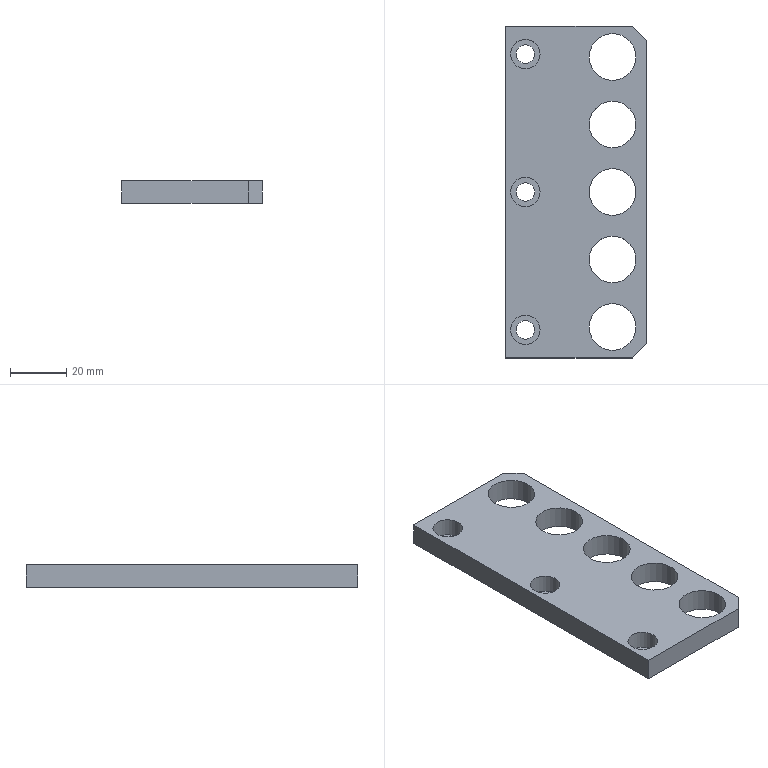NC program | NX | posted with a generic post | part box 50 x 118 x 8 mm
Whole program:
N10 G17 G21 G94 G90
(PLANAR_MILL_6 , TOOL : D63R0.8)
N12 T01 M6
N14 G54
N16 G17 G0 G90 X98.825 Y0.176 S2500 M3
N18 G43 Z30. H1
N20 Z5.7
N22 G94 G1 Z3.7 F800.
N24 X62.5
N26 X-62.5
N28 X-98.825
N30 Z5.7
N32 G0 Z30.
N34 X98.975 Y0.025
N36 Z5.4
N38 G1 Z3.4
N40 X62.5
N42 X-62.5
N44 X-98.975
N46 Z5.4
N48 G0 Z30.
N50 X99. Y0.
N52 Z5.1
N54 G1 Z3.1
N56 X62.5
N58 X-62.5
N60 X-99.
N62 Z5.1
N64 G0 Z30.
N66 X99.
N68 Z4.8
N70 G1 Z2.8
N72 X62.5
N74 X-62.5
N76 X-99.
N78 Z4.8
N80 G0 Z30.
N82 X99.
N84 Z4.5
N86 G1 Z2.5
N88 X62.5
N90 X-62.5
N92 X-99.
N94 Z4.5
N96 G0 Z30.
N98 X99.
N100 Z4.2
N102 G1 Z2.2
N104 X62.5
N106 X-62.5
N108 X-99.
N110 Z4.2
N112 G0 Z30.
N114 X99.
N116 Z3.9
N118 G1 Z1.9
N120 X62.5
N122 X-62.5
N124 X-99.
N126 Z3.9
N128 G0 Z30.
N130 X99.
N132 Z3.6
N134 G1 Z1.6
N136 X62.5
N138 X-62.5
N140 X-99.
N142 Z3.6
N144 G0 Z30.
N146 X99.
N148 Z3.3
N150 G1 Z1.3
N152 X62.5
N154 X-62.5
N156 X-99.
N158 Z3.3
N160 G0 Z30.
N162 X99.
N164 Z3.
N166 G1 Z1.
N168 X62.5
N170 X-62.5
N172 X-99.
N174 Z3.
N176 G0 Z30.
N178 X99.
N180 Z2.7
N182 G1 Z0.7
N184 X62.5
N186 X-62.5
N188 X-99.
N190 Z2.7
N192 G0 Z30.
N194 X99.
N196 Z2.4
N198 G1 Z0.4
N200 X62.5
N202 X-62.5
N204 X-99.
N206 Z2.4
N208 G0 Z30.
N210 X99.
N212 Z2.1
N214 G1 Z0.1
N216 X62.5
N218 X-62.5
N220 X-99.
N222 Z2.1
N224 G0 Z30.
(PLANAR_MILL_6_COPY , TOOL : D63R0.8)
N226 X99.
N228 Z2.
N230 G1 Z0.
N232 X62.5
N234 X-62.5
N236 X-99.
N238 Z2.
N240 G0 Z30.
N242 M5
(PLANAR_MILL_7 , TOOL : D4点钻)
N244 T05 M6
N246 G54
N248 G17 G0 G90 X61.828 Y-26. S3000 M3
N250 G43 Z30. H5
N252 Z2.
N254 G94 G1 Z-1. F800.
N256 X58.999
N258 X-59.
N260 G2 X-60. Y-25. R1.
N262 G1 Y20.
N264 G2 X-59.707 Y20.707 R1.
N266 G1 X-54.707 Y25.707
N268 G2 X-54. Y26. R1.
N270 G1 X54.
N272 G2 X54.707 Y25.707 R1.
N274 G1 X59.707 Y20.707
N276 G2 X60. Y20. R1.
N278 G1 Y-24.999
N280 Y-27.828
N282 Z2.
N284 G0 Z30.
(PLANAR_MILL_8 , TOOL : D4点钻)
N286 X50. Y-17.169
N288 Z1.
N290 G1 Z-1.
N292 Y-16.7
N294 G3 X49. Y-15.7 R1.
N296 X46.7 Y-18. R2.3
N298 X49. Y-15.7 R-2.3
N300 X48. Y-16.7 R1.
N302 G1 Y-17.169
N304 Z1.
N306 G0 Z30.
N308 X49. Y19.22
N310 Z1.
N312 G1 Z-1.
N314 Y19.3
N316 G3 X48. Y20.3 R1.
N318 X40.7 Y13. R7.3
N320 X48. Y20.3 R-7.3
N322 X47. Y19.3 R1.
N324 G1 Y19.22
N326 Z1.
N328 G0 Z30.
N330 X25.
N332 Z1.
N334 G1 Z-1.
N336 Y19.3
N338 G3 X24. Y20.3 R1.
N340 X16.7 Y13. R7.3
N342 X24. Y20.3 R-7.3
N344 X23. Y19.3 R1.
N346 G1 Y19.22
N348 Z1.
N350 G0 Z30.
N352 X1. Y-17.169
N354 Z1.
N356 G1 Z-1.
N358 Y-16.7
N360 G3 X0. Y-15.7 R1.
N362 X-2.3 Y-18. R2.3
N364 X0. Y-15.7 R-2.3
N366 X-1. Y-16.7 R1.
N368 G1 Y-17.169
N370 Z1.
N372 G0 Z30.
N374 X1. Y19.22
N376 Z1.
N378 G1 Z-1.
N380 Y19.3
N382 G3 X0. Y20.3 R1.
N384 X-7.3 Y13. R7.3
N386 X0. Y20.3 R-7.3
N388 X-1. Y19.3 R1.
N390 G1 Y19.22
N392 Z1.
N394 G0 Z30.
N396 X-23.
N398 Z1.
N400 G1 Z-1.
N402 Y19.3
N404 G3 X-24. Y20.3 R1.
N406 X-31.3 Y13. R7.3
N408 X-24. Y20.3 R-7.3
N410 X-25. Y19.3 R1.
N412 G1 Y19.22
N414 Z1.
N416 G0 Z30.
N418 X-47.
N420 Z1.
N422 G1 Z-1.
N424 Y19.3
N426 G3 X-48. Y20.3 R1.
N428 X-55.3 Y13. R7.3
N430 X-48. Y20.3 R-7.3
N432 X-49. Y19.3 R1.
N434 G1 Y19.22
N436 Z1.
N438 G0 Z30.
N440 X-48. Y-17.169
N442 Z1.
N444 G1 Z-1.
N446 Y-16.7
N448 G3 X-49. Y-15.7 R1.
N450 X-51.3 Y-18. R2.3
N452 X-49. Y-15.7 R-2.3
N454 X-50. Y-16.7 R1.
N456 G1 Y-17.169
N458 Z1.
N460 G0 Z30.
N462 M5
N464 M2